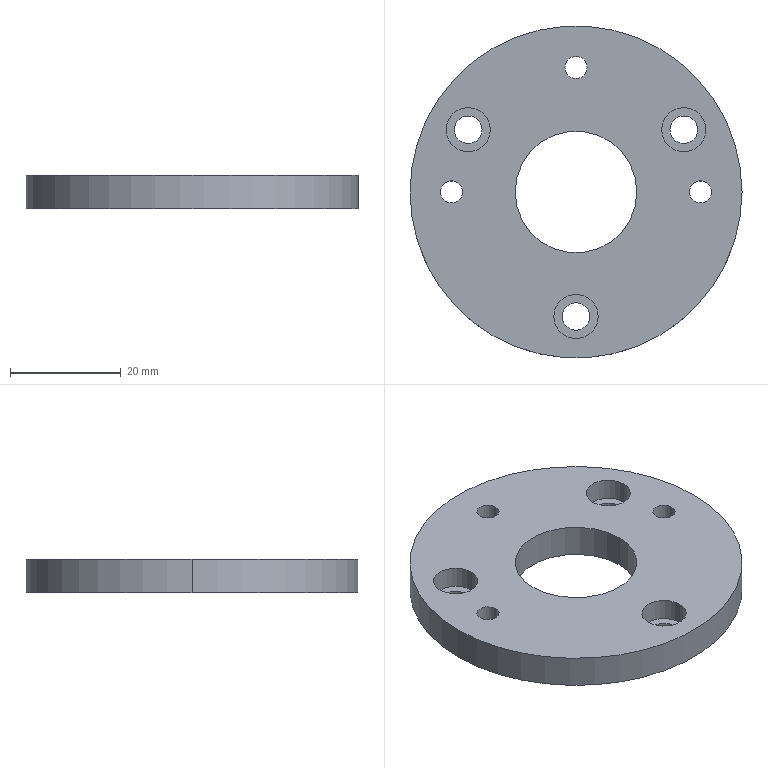Part | SolidWorks | features FlatPattern 1, ICE 1, SMBaseFlange 1, SheetMetal 1 | 1 solid | 27 faces | box 60 x 60 x 6 mm | volume 13737 mm3 | cylinder 22 | plane 5 | commonest cylinder face diameters 4 x6 5 x6 8 x6 22 x2 60 x2
STEP:
#1=CARTESIAN_POINT('',(1118.202,163.897,-4.));
#2=VERTEX_POINT('',#1);
#3=CARTESIAN_POINT('',(1126.202,163.897,-4.));
#4=VERTEX_POINT('',#3);
#5=CARTESIAN_POINT('',(1122.202,163.897,-4.));
#6=DIRECTION('',(0.,0.,1.));
#7=DIRECTION('',(1.,0.,0.));
#8=AXIS2_PLACEMENT_3D('',#5,#6,#7);
#9=CIRCLE('',#8,4.);
#10=EDGE_CURVE('',#2,#4,#9,.T.);
#11=ORIENTED_EDGE('',*,*,#10,.F.);
#12=CARTESIAN_POINT('',(1118.202,163.897,0.));
#13=VERTEX_POINT('',#12);
#14=CARTESIAN_POINT('',(1118.202,163.897,-4.));
#15=DIRECTION('',(0.,0.,1.));
#16=VECTOR('',#15,1000.);
#17=LINE('',#14,#16);
#18=EDGE_CURVE('',#2,#13,#17,.T.);
#19=ORIENTED_EDGE('',*,*,#18,.T.);
#20=CARTESIAN_POINT('',(1126.202,163.897,0.));
#21=VERTEX_POINT('',#20);
#22=CARTESIAN_POINT('',(1122.202,163.897,0.));
#23=DIRECTION('',(0.,0.,1.));
#24=DIRECTION('',(1.,0.,0.));
#25=AXIS2_PLACEMENT_3D('',#22,#23,#24);
#26=CIRCLE('',#25,4.);
#27=EDGE_CURVE('',#13,#21,#26,.T.);
#28=ORIENTED_EDGE('',*,*,#27,.T.);
#29=CARTESIAN_POINT('',(1126.202,163.897,-4.));
#30=DIRECTION('',(0.,0.,1.));
#31=VECTOR('',#30,1000.);
#32=LINE('',#29,#31);
#33=EDGE_CURVE('',#4,#21,#32,.T.);
#34=ORIENTED_EDGE('',*,*,#33,.F.);
#35=EDGE_LOOP('',(#11,#19,#28,#34));
#36=FACE_OUTER_BOUND('',#35,.T.);
#37=CARTESIAN_POINT('',(1122.202,163.897,-4.));
#38=DIRECTION('',(0.,0.,1.));
#39=DIRECTION('',(1.,0.,0.));
#40=AXIS2_PLACEMENT_3D('',#37,#38,#39);
#41=CYLINDRICAL_SURFACE('',#40,4.);
#42=ADVANCED_FACE('',(#36),#41,.F.);
#43=CARTESIAN_POINT('',(1137.687,197.647,-4.));
#44=VERTEX_POINT('',#43);
#45=CARTESIAN_POINT('',(1145.687,197.647,-4.));
#46=VERTEX_POINT('',#45);
#47=CARTESIAN_POINT('',(1141.687,197.647,-4.));
#48=DIRECTION('',(0.,0.,1.));
#49=DIRECTION('',(1.,0.,0.));
#50=AXIS2_PLACEMENT_3D('',#47,#48,#49);
#51=CIRCLE('',#50,4.);
#52=EDGE_CURVE('',#44,#46,#51,.T.);
#53=ORIENTED_EDGE('',*,*,#52,.F.);
#54=CARTESIAN_POINT('',(1137.687,197.647,0.));
#55=VERTEX_POINT('',#54);
#56=CARTESIAN_POINT('',(1137.687,197.647,-4.));
#57=DIRECTION('',(0.,0.,1.));
#58=VECTOR('',#57,1000.);
#59=LINE('',#56,#58);
#60=EDGE_CURVE('',#44,#55,#59,.T.);
#61=ORIENTED_EDGE('',*,*,#60,.T.);
#62=CARTESIAN_POINT('',(1145.687,197.647,0.));
#63=VERTEX_POINT('',#62);
#64=CARTESIAN_POINT('',(1141.687,197.647,0.));
#65=DIRECTION('',(0.,0.,1.));
#66=DIRECTION('',(1.,0.,0.));
#67=AXIS2_PLACEMENT_3D('',#64,#65,#66);
#68=CIRCLE('',#67,4.);
#69=EDGE_CURVE('',#55,#63,#68,.T.);
#70=ORIENTED_EDGE('',*,*,#69,.T.);
#71=CARTESIAN_POINT('',(1145.687,197.647,-4.));
#72=DIRECTION('',(0.,0.,1.));
#73=VECTOR('',#72,1000.);
#74=LINE('',#71,#73);
#75=EDGE_CURVE('',#46,#63,#74,.T.);
#76=ORIENTED_EDGE('',*,*,#75,.F.);
#77=EDGE_LOOP('',(#53,#61,#70,#76));
#78=FACE_OUTER_BOUND('',#77,.T.);
#79=CARTESIAN_POINT('',(1141.687,197.647,-4.));
#80=DIRECTION('',(0.,0.,1.));
#81=DIRECTION('',(1.,0.,0.));
#82=AXIS2_PLACEMENT_3D('',#79,#80,#81);
#83=CYLINDRICAL_SURFACE('',#82,4.);
#84=ADVANCED_FACE('',(#78),#83,.F.);
#85=CARTESIAN_POINT('',(1098.716,197.647,-4.));
#86=VERTEX_POINT('',#85);
#87=CARTESIAN_POINT('',(1106.716,197.647,-4.));
#88=VERTEX_POINT('',#87);
#89=CARTESIAN_POINT('',(1102.716,197.647,-4.));
#90=DIRECTION('',(0.,0.,1.));
#91=DIRECTION('',(1.,0.,0.));
#92=AXIS2_PLACEMENT_3D('',#89,#90,#91);
#93=CIRCLE('',#92,4.);
#94=EDGE_CURVE('',#86,#88,#93,.T.);
#95=ORIENTED_EDGE('',*,*,#94,.F.);
#96=CARTESIAN_POINT('',(1098.716,197.647,0.));
#97=VERTEX_POINT('',#96);
#98=CARTESIAN_POINT('',(1098.716,197.647,-4.));
#99=DIRECTION('',(0.,0.,1.));
#100=VECTOR('',#99,1000.);
#101=LINE('',#98,#100);
#102=EDGE_CURVE('',#86,#97,#101,.T.);
#103=ORIENTED_EDGE('',*,*,#102,.T.);
#104=CARTESIAN_POINT('',(1106.716,197.647,0.));
#105=VERTEX_POINT('',#104);
#106=CARTESIAN_POINT('',(1102.716,197.647,0.));
#107=DIRECTION('',(0.,0.,1.));
#108=DIRECTION('',(1.,0.,0.));
#109=AXIS2_PLACEMENT_3D('',#106,#107,#108);
#110=CIRCLE('',#109,4.);
#111=EDGE_CURVE('',#97,#105,#110,.T.);
#112=ORIENTED_EDGE('',*,*,#111,.T.);
#113=CARTESIAN_POINT('',(1106.716,197.647,-4.));
#114=DIRECTION('',(0.,0.,1.));
#115=VECTOR('',#114,1000.);
#116=LINE('',#113,#115);
#117=EDGE_CURVE('',#88,#105,#116,.T.);
#118=ORIENTED_EDGE('',*,*,#117,.F.);
#119=EDGE_LOOP('',(#95,#103,#112,#118));
#120=FACE_OUTER_BOUND('',#119,.T.);
#121=CARTESIAN_POINT('',(1102.716,197.647,-4.));
#122=DIRECTION('',(0.,0.,1.));
#123=DIRECTION('',(1.,0.,0.));
#124=AXIS2_PLACEMENT_3D('',#121,#122,#123);
#125=CYLINDRICAL_SURFACE('',#124,4.);
#126=ADVANCED_FACE('',(#120),#125,.F.);
#127=CARTESIAN_POINT('',(1142.702,186.397,-6.));
#128=VERTEX_POINT('',#127);
#129=CARTESIAN_POINT('',(1146.702,186.397,-6.));
#130=VERTEX_POINT('',#129);
#131=CARTESIAN_POINT('',(1144.702,186.397,-6.));
#132=DIRECTION('',(0.,0.,1.));
#133=DIRECTION('',(1.,0.,0.));
#134=AXIS2_PLACEMENT_3D('',#131,#132,#133);
#135=CIRCLE('',#134,2.);
#136=EDGE_CURVE('',#128,#130,#135,.T.);
#137=ORIENTED_EDGE('',*,*,#136,.F.);
#138=CARTESIAN_POINT('',(1142.702,186.397,0.));
#139=VERTEX_POINT('',#138);
#140=CARTESIAN_POINT('',(1142.702,186.397,-6.));
#141=DIRECTION('',(0.,0.,1.));
#142=VECTOR('',#141,1000.);
#143=LINE('',#140,#142);
#144=EDGE_CURVE('',#128,#139,#143,.T.);
#145=ORIENTED_EDGE('',*,*,#144,.T.);
#146=CARTESIAN_POINT('',(1146.702,186.397,0.));
#147=VERTEX_POINT('',#146);
#148=CARTESIAN_POINT('',(1144.702,186.397,0.));
#149=DIRECTION('',(0.,0.,1.));
#150=DIRECTION('',(1.,0.,0.));
#151=AXIS2_PLACEMENT_3D('',#148,#149,#150);
#152=CIRCLE('',#151,2.);
#153=EDGE_CURVE('',#139,#147,#152,.T.);
#154=ORIENTED_EDGE('',*,*,#153,.T.);
#155=CARTESIAN_POINT('',(1146.702,186.397,-6.));
#156=DIRECTION('',(0.,0.,1.));
#157=VECTOR('',#156,1000.);
#158=LINE('',#155,#157);
#159=EDGE_CURVE('',#130,#147,#158,.T.);
#160=ORIENTED_EDGE('',*,*,#159,.F.);
#161=EDGE_LOOP('',(#137,#145,#154,#160));
#162=FACE_OUTER_BOUND('',#161,.T.);
#163=CARTESIAN_POINT('',(1144.702,186.397,-6.));
#164=DIRECTION('',(0.,0.,1.));
#165=DIRECTION('',(1.,0.,0.));
#166=AXIS2_PLACEMENT_3D('',#163,#164,#165);
#167=CYLINDRICAL_SURFACE('',#166,2.);
#168=ADVANCED_FACE('',(#162),#167,.F.);
#169=CARTESIAN_POINT('',(1097.702,186.397,-6.));
#170=VERTEX_POINT('',#169);
#171=CARTESIAN_POINT('',(1101.702,186.397,-6.));
#172=VERTEX_POINT('',#171);
#173=CARTESIAN_POINT('',(1099.702,186.397,-6.));
#174=DIRECTION('',(0.,0.,1.));
#175=DIRECTION('',(1.,0.,0.));
#176=AXIS2_PLACEMENT_3D('',#173,#174,#175);
#177=CIRCLE('',#176,2.);
#178=EDGE_CURVE('',#170,#172,#177,.T.);
#179=ORIENTED_EDGE('',*,*,#178,.F.);
#180=CARTESIAN_POINT('',(1097.702,186.397,0.));
#181=VERTEX_POINT('',#180);
#182=CARTESIAN_POINT('',(1097.702,186.397,-6.));
#183=DIRECTION('',(0.,0.,1.));
#184=VECTOR('',#183,1000.);
#185=LINE('',#182,#184);
#186=EDGE_CURVE('',#170,#181,#185,.T.);
#187=ORIENTED_EDGE('',*,*,#186,.T.);
#188=CARTESIAN_POINT('',(1101.702,186.397,0.));
#189=VERTEX_POINT('',#188);
#190=CARTESIAN_POINT('',(1099.702,186.397,0.));
#191=DIRECTION('',(0.,0.,1.));
#192=DIRECTION('',(1.,0.,0.));
#193=AXIS2_PLACEMENT_3D('',#190,#191,#192);
#194=CIRCLE('',#193,2.);
#195=EDGE_CURVE('',#181,#189,#194,.T.);
#196=ORIENTED_EDGE('',*,*,#195,.T.);
#197=CARTESIAN_POINT('',(1101.702,186.397,-6.));
#198=DIRECTION('',(0.,0.,1.));
#199=VECTOR('',#198,1000.);
#200=LINE('',#197,#199);
#201=EDGE_CURVE('',#172,#189,#200,.T.);
#202=ORIENTED_EDGE('',*,*,#201,.F.);
#203=EDGE_LOOP('',(#179,#187,#196,#202));
#204=FACE_OUTER_BOUND('',#203,.T.);
#205=CARTESIAN_POINT('',(1099.702,186.397,-6.));
#206=DIRECTION('',(0.,0.,1.));
#207=DIRECTION('',(1.,0.,0.));
#208=AXIS2_PLACEMENT_3D('',#205,#206,#207);
#209=CYLINDRICAL_SURFACE('',#208,2.);
#210=ADVANCED_FACE('',(#204),#209,.F.);
#211=CARTESIAN_POINT('',(1111.202,186.397,-6.));
#212=VERTEX_POINT('',#211);
#213=CARTESIAN_POINT('',(1133.202,186.397,-6.));
#214=VERTEX_POINT('',#213);
#215=CARTESIAN_POINT('',(1122.202,186.397,-6.));
#216=DIRECTION('',(0.,0.,1.));
#217=DIRECTION('',(1.,0.,0.));
#218=AXIS2_PLACEMENT_3D('',#215,#216,#217);
#219=CIRCLE('',#218,11.);
#220=EDGE_CURVE('',#212,#214,#219,.T.);
#221=ORIENTED_EDGE('',*,*,#220,.F.);
#222=CARTESIAN_POINT('',(1111.202,186.397,0.));
#223=VERTEX_POINT('',#222);
#224=CARTESIAN_POINT('',(1111.202,186.397,-6.));
#225=DIRECTION('',(0.,0.,1.));
#226=VECTOR('',#225,1000.);
#227=LINE('',#224,#226);
#228=EDGE_CURVE('',#212,#223,#227,.T.);
#229=ORIENTED_EDGE('',*,*,#228,.T.);
#230=CARTESIAN_POINT('',(1133.202,186.397,0.));
#231=VERTEX_POINT('',#230);
#232=CARTESIAN_POINT('',(1122.202,186.397,0.));
#233=DIRECTION('',(0.,0.,1.));
#234=DIRECTION('',(1.,0.,0.));
#235=AXIS2_PLACEMENT_3D('',#232,#233,#234);
#236=CIRCLE('',#235,11.);
#237=EDGE_CURVE('',#223,#231,#236,.T.);
#238=ORIENTED_EDGE('',*,*,#237,.T.);
#239=CARTESIAN_POINT('',(1133.202,186.397,-6.));
#240=DIRECTION('',(0.,0.,1.));
#241=VECTOR('',#240,1000.);
#242=LINE('',#239,#241);
#243=EDGE_CURVE('',#214,#231,#242,.T.);
#244=ORIENTED_EDGE('',*,*,#243,.F.);
#245=EDGE_LOOP('',(#221,#229,#238,#244));
#246=FACE_OUTER_BOUND('',#245,.T.);
#247=CARTESIAN_POINT('',(1122.202,186.397,-6.));
#248=DIRECTION('',(0.,0.,1.));
#249=DIRECTION('',(1.,0.,0.));
#250=AXIS2_PLACEMENT_3D('',#247,#248,#249);
#251=CYLINDRICAL_SURFACE('',#250,11.);
#252=ADVANCED_FACE('',(#246),#251,.F.);
#253=CARTESIAN_POINT('',(1120.202,208.897,-6.));
#254=VERTEX_POINT('',#253);
#255=CARTESIAN_POINT('',(1124.202,208.897,-6.));
#256=VERTEX_POINT('',#255);
#257=CARTESIAN_POINT('',(1122.202,208.897,-6.));
#258=DIRECTION('',(0.,0.,1.));
#259=DIRECTION('',(1.,0.,0.));
#260=AXIS2_PLACEMENT_3D('',#257,#258,#259);
#261=CIRCLE('',#260,2.);
#262=EDGE_CURVE('',#254,#256,#261,.T.);
#263=ORIENTED_EDGE('',*,*,#262,.F.);
#264=CARTESIAN_POINT('',(1120.202,208.897,0.));
#265=VERTEX_POINT('',#264);
#266=CARTESIAN_POINT('',(1120.202,208.897,-6.));
#267=DIRECTION('',(0.,0.,1.));
#268=VECTOR('',#267,1000.);
#269=LINE('',#266,#268);
#270=EDGE_CURVE('',#254,#265,#269,.T.);
#271=ORIENTED_EDGE('',*,*,#270,.T.);
#272=CARTESIAN_POINT('',(1124.202,208.897,0.));
#273=VERTEX_POINT('',#272);
#274=CARTESIAN_POINT('',(1122.202,208.897,0.));
#275=DIRECTION('',(0.,0.,1.));
#276=DIRECTION('',(1.,0.,0.));
#277=AXIS2_PLACEMENT_3D('',#274,#275,#276);
#278=CIRCLE('',#277,2.);
#279=EDGE_CURVE('',#265,#273,#278,.T.);
#280=ORIENTED_EDGE('',*,*,#279,.T.);
#281=CARTESIAN_POINT('',(1124.202,208.897,-6.));
#282=DIRECTION('',(0.,0.,1.));
#283=VECTOR('',#282,1000.);
#284=LINE('',#281,#283);
#285=EDGE_CURVE('',#256,#273,#284,.T.);
#286=ORIENTED_EDGE('',*,*,#285,.F.);
#287=EDGE_LOOP('',(#263,#271,#280,#286));
#288=FACE_OUTER_BOUND('',#287,.T.);
#289=CARTESIAN_POINT('',(1122.202,208.897,-6.));
#290=DIRECTION('',(0.,0.,1.));
#291=DIRECTION('',(1.,0.,0.));
#292=AXIS2_PLACEMENT_3D('',#289,#290,#291);
#293=CYLINDRICAL_SURFACE('',#292,2.);
#294=ADVANCED_FACE('',(#288),#293,.F.);
#295=CARTESIAN_POINT('',(1152.202,186.397,-6.));
#296=VERTEX_POINT('',#295);
#297=CARTESIAN_POINT('',(1092.202,186.397,-6.));
#298=VERTEX_POINT('',#297);
#299=CARTESIAN_POINT('',(1122.202,186.397,-6.));
#300=DIRECTION('',(0.,0.,1.));
#301=DIRECTION('',(1.,0.,0.));
#302=AXIS2_PLACEMENT_3D('',#299,#300,#301);
#303=CIRCLE('',#302,30.);
#304=EDGE_CURVE('',#296,#298,#303,.T.);
#305=ORIENTED_EDGE('',*,*,#304,.T.);
#306=CARTESIAN_POINT('',(1092.202,186.397,0.));
#307=VERTEX_POINT('',#306);
#308=CARTESIAN_POINT('',(1092.202,186.397,-6.));
#309=DIRECTION('',(0.,0.,1.));
#310=VECTOR('',#309,1000.);
#311=LINE('',#308,#310);
#312=EDGE_CURVE('',#298,#307,#311,.T.);
#313=ORIENTED_EDGE('',*,*,#312,.T.);
#314=CARTESIAN_POINT('',(1152.202,186.397,0.));
#315=VERTEX_POINT('',#314);
#316=CARTESIAN_POINT('',(1122.202,186.397,0.));
#317=DIRECTION('',(0.,0.,1.));
#318=DIRECTION('',(1.,0.,0.));
#319=AXIS2_PLACEMENT_3D('',#316,#317,#318);
#320=CIRCLE('',#319,30.);
#321=EDGE_CURVE('',#315,#307,#320,.T.);
#322=ORIENTED_EDGE('',*,*,#321,.F.);
#323=CARTESIAN_POINT('',(1152.202,186.397,-6.));
#324=DIRECTION('',(0.,0.,1.));
#325=VECTOR('',#324,1000.);
#326=LINE('',#323,#325);
#327=EDGE_CURVE('',#296,#315,#326,.T.);
#328=ORIENTED_EDGE('',*,*,#327,.F.);
#329=EDGE_LOOP('',(#305,#313,#322,#328));
#330=FACE_OUTER_BOUND('',#329,.T.);
#331=CARTESIAN_POINT('',(1122.202,186.397,-6.));
#332=DIRECTION('',(0.,0.,1.));
#333=DIRECTION('',(1.,0.,0.));
#334=AXIS2_PLACEMENT_3D('',#331,#332,#333);
#335=CYLINDRICAL_SURFACE('',#334,30.);
#336=ADVANCED_FACE('',(#330),#335,.T.);
#337=CARTESIAN_POINT('',(1100.216,197.647,-6.));
#338=VERTEX_POINT('',#337);
#339=CARTESIAN_POINT('',(1105.216,197.647,-6.));
#340=VERTEX_POINT('',#339);
#341=CARTESIAN_POINT('',(1102.716,197.647,-6.));
#342=DIRECTION('',(0.,0.,1.));
#343=DIRECTION('',(1.,0.,0.));
#344=AXIS2_PLACEMENT_3D('',#341,#342,#343);
#345=CIRCLE('',#344,2.5);
#346=EDGE_CURVE('',#338,#340,#345,.T.);
#347=ORIENTED_EDGE('',*,*,#346,.F.);
#348=CARTESIAN_POINT('',(1100.216,197.647,-4.));
#349=VERTEX_POINT('',#348);
#350=CARTESIAN_POINT('',(1100.216,197.647,-6.));
#351=DIRECTION('',(0.,0.,1.));
#352=VECTOR('',#351,1000.);
#353=LINE('',#350,#352);
#354=EDGE_CURVE('',#338,#349,#353,.T.);
#355=ORIENTED_EDGE('',*,*,#354,.T.);
#356=CARTESIAN_POINT('',(1105.216,197.647,-4.));
#357=VERTEX_POINT('',#356);
#358=CARTESIAN_POINT('',(1102.716,197.647,-4.));
#359=DIRECTION('',(0.,0.,-1.));
#360=DIRECTION('',(1.,0.,0.));
#361=AXIS2_PLACEMENT_3D('',#358,#359,#360);
#362=CIRCLE('',#361,2.5);
#363=EDGE_CURVE('',#357,#349,#362,.T.);
#364=ORIENTED_EDGE('',*,*,#363,.F.);
#365=CARTESIAN_POINT('',(1105.216,197.647,-6.));
#366=DIRECTION('',(0.,0.,1.));
#367=VECTOR('',#366,1000.);
#368=LINE('',#365,#367);
#369=EDGE_CURVE('',#340,#357,#368,.T.);
#370=ORIENTED_EDGE('',*,*,#369,.F.);
#371=EDGE_LOOP('',(#347,#355,#364,#370));
#372=FACE_OUTER_BOUND('',#371,.T.);
#373=CARTESIAN_POINT('',(1102.716,197.647,-6.));
#374=DIRECTION('',(0.,0.,1.));
#375=DIRECTION('',(1.,0.,0.));
#376=AXIS2_PLACEMENT_3D('',#373,#374,#375);
#377=CYLINDRICAL_SURFACE('',#376,2.5);
#378=ADVANCED_FACE('',(#372),#377,.F.);
#379=CARTESIAN_POINT('',(1139.187,197.647,-6.));
#380=VERTEX_POINT('',#379);
#381=CARTESIAN_POINT('',(1144.187,197.647,-6.));
#382=VERTEX_POINT('',#381);
#383=CARTESIAN_POINT('',(1141.687,197.647,-6.));
#384=DIRECTION('',(0.,0.,1.));
#385=DIRECTION('',(1.,0.,0.));
#386=AXIS2_PLACEMENT_3D('',#383,#384,#385);
#387=CIRCLE('',#386,2.5);
#388=EDGE_CURVE('',#380,#382,#387,.T.);
#389=ORIENTED_EDGE('',*,*,#388,.F.);
#390=CARTESIAN_POINT('',(1139.187,197.647,-4.));
#391=VERTEX_POINT('',#390);
#392=CARTESIAN_POINT('',(1139.187,197.647,-6.));
#393=DIRECTION('',(0.,0.,1.));
#394=VECTOR('',#393,1000.);
#395=LINE('',#392,#394);
#396=EDGE_CURVE('',#380,#391,#395,.T.);
#397=ORIENTED_EDGE('',*,*,#396,.T.);
#398=CARTESIAN_POINT('',(1144.187,197.647,-4.));
#399=VERTEX_POINT('',#398);
#400=CARTESIAN_POINT('',(1141.687,197.647,-4.));
#401=DIRECTION('',(0.,0.,-1.));
#402=DIRECTION('',(1.,0.,0.));
#403=AXIS2_PLACEMENT_3D('',#400,#401,#402);
#404=CIRCLE('',#403,2.5);
#405=EDGE_CURVE('',#399,#391,#404,.T.);
#406=ORIENTED_EDGE('',*,*,#405,.F.);
#407=CARTESIAN_POINT('',(1144.187,197.647,-6.));
#408=DIRECTION('',(0.,0.,1.));
#409=VECTOR('',#408,1000.);
#410=LINE('',#407,#409);
#411=EDGE_CURVE('',#382,#399,#410,.T.);
#412=ORIENTED_EDGE('',*,*,#411,.F.);
#413=EDGE_LOOP('',(#389,#397,#406,#412));
#414=FACE_OUTER_BOUND('',#413,.T.);
#415=CARTESIAN_POINT('',(1141.687,197.647,-6.));
#416=DIRECTION('',(0.,0.,1.));
#417=DIRECTION('',(1.,0.,0.));
#418=AXIS2_PLACEMENT_3D('',#415,#416,#417);
#419=CYLINDRICAL_SURFACE('',#418,2.5);
#420=ADVANCED_FACE('',(#414),#419,.F.);
#421=CARTESIAN_POINT('',(1119.702,163.897,-6.));
#422=VERTEX_POINT('',#421);
#423=CARTESIAN_POINT('',(1124.702,163.897,-6.));
#424=VERTEX_POINT('',#423);
#425=CARTESIAN_POINT('',(1122.202,163.897,-6.));
#426=DIRECTION('',(0.,0.,1.));
#427=DIRECTION('',(1.,0.,0.));
#428=AXIS2_PLACEMENT_3D('',#425,#426,#427);
#429=CIRCLE('',#428,2.5);
#430=EDGE_CURVE('',#422,#424,#429,.T.);
#431=ORIENTED_EDGE('',*,*,#430,.F.);
#432=CARTESIAN_POINT('',(1119.702,163.897,-4.));
#433=VERTEX_POINT('',#432);
#434=CARTESIAN_POINT('',(1119.702,163.897,-6.));
#435=DIRECTION('',(0.,0.,1.));
#436=VECTOR('',#435,1000.);
#437=LINE('',#434,#436);
#438=EDGE_CURVE('',#422,#433,#437,.T.);
#439=ORIENTED_EDGE('',*,*,#438,.T.);
#440=CARTESIAN_POINT('',(1124.702,163.897,-4.));
#441=VERTEX_POINT('',#440);
#442=CARTESIAN_POINT('',(1122.202,163.897,-4.));
#443=DIRECTION('',(0.,0.,-1.));
#444=DIRECTION('',(1.,0.,0.));
#445=AXIS2_PLACEMENT_3D('',#442,#443,#444);
#446=CIRCLE('',#445,2.5);
#447=EDGE_CURVE('',#441,#433,#446,.T.);
#448=ORIENTED_EDGE('',*,*,#447,.F.);
#449=CARTESIAN_POINT('',(1124.702,163.897,-6.));
#450=DIRECTION('',(0.,0.,1.));
#451=VECTOR('',#450,1000.);
#452=LINE('',#449,#451);
#453=EDGE_CURVE('',#424,#441,#452,.T.);
#454=ORIENTED_EDGE('',*,*,#453,.F.);
#455=EDGE_LOOP('',(#431,#439,#448,#454));
#456=FACE_OUTER_BOUND('',#455,.T.);
#457=CARTESIAN_POINT('',(1122.202,163.897,-6.));
#458=DIRECTION('',(0.,0.,1.));
#459=DIRECTION('',(1.,0.,0.));
#460=AXIS2_PLACEMENT_3D('',#457,#458,#459);
#461=CYLINDRICAL_SURFACE('',#460,2.5);
#462=ADVANCED_FACE('',(#456),#461,.F.);
#463=ORIENTED_EDGE('',*,*,#438,.F.);
#464=CARTESIAN_POINT('',(1122.202,163.897,-6.));
#465=DIRECTION('',(0.,0.,1.));
#466=DIRECTION('',(1.,0.,0.));
#467=AXIS2_PLACEMENT_3D('',#464,#465,#466);
#468=CIRCLE('',#467,2.5);
#469=EDGE_CURVE('',#424,#422,#468,.T.);
#470=ORIENTED_EDGE('',*,*,#469,.F.);
#471=ORIENTED_EDGE('',*,*,#453,.T.);
#472=CARTESIAN_POINT('',(1122.202,163.897,-4.));
#473=DIRECTION('',(0.,0.,-1.));
#474=DIRECTION('',(1.,0.,0.));
#475=AXIS2_PLACEMENT_3D('',#472,#473,#474);
#476=CIRCLE('',#475,2.5);
#477=EDGE_CURVE('',#433,#441,#476,.T.);
#478=ORIENTED_EDGE('',*,*,#477,.F.);
#479=EDGE_LOOP('',(#463,#470,#471,#478));
#480=FACE_OUTER_BOUND('',#479,.T.);
#481=CARTESIAN_POINT('',(1122.202,163.897,-6.));
#482=DIRECTION('',(0.,0.,1.));
#483=DIRECTION('',(1.,0.,0.));
#484=AXIS2_PLACEMENT_3D('',#481,#482,#483);
#485=CYLINDRICAL_SURFACE('',#484,2.5);
#486=ADVANCED_FACE('',(#480),#485,.F.);
#487=ORIENTED_EDGE('',*,*,#396,.F.);
#488=CARTESIAN_POINT('',(1141.687,197.647,-6.));
#489=DIRECTION('',(0.,0.,1.));
#490=DIRECTION('',(1.,0.,0.));
#491=AXIS2_PLACEMENT_3D('',#488,#489,#490);
#492=CIRCLE('',#491,2.5);
#493=EDGE_CURVE('',#382,#380,#492,.T.);
#494=ORIENTED_EDGE('',*,*,#493,.F.);
#495=ORIENTED_EDGE('',*,*,#411,.T.);
#496=CARTESIAN_POINT('',(1141.687,197.647,-4.));
#497=DIRECTION('',(0.,0.,-1.));
#498=DIRECTION('',(1.,0.,0.));
#499=AXIS2_PLACEMENT_3D('',#496,#497,#498);
#500=CIRCLE('',#499,2.5);
#501=EDGE_CURVE('',#391,#399,#500,.T.);
#502=ORIENTED_EDGE('',*,*,#501,.F.);
#503=EDGE_LOOP('',(#487,#494,#495,#502));
#504=FACE_OUTER_BOUND('',#503,.T.);
#505=CARTESIAN_POINT('',(1141.687,197.647,-6.));
#506=DIRECTION('',(0.,0.,1.));
#507=DIRECTION('',(1.,0.,0.));
#508=AXIS2_PLACEMENT_3D('',#505,#506,#507);
#509=CYLINDRICAL_SURFACE('',#508,2.5);
#510=ADVANCED_FACE('',(#504),#509,.F.);
#511=ORIENTED_EDGE('',*,*,#354,.F.);
#512=CARTESIAN_POINT('',(1102.716,197.647,-6.));
#513=DIRECTION('',(0.,0.,1.));
#514=DIRECTION('',(1.,0.,0.));
#515=AXIS2_PLACEMENT_3D('',#512,#513,#514);
#516=CIRCLE('',#515,2.5);
#517=EDGE_CURVE('',#340,#338,#516,.T.);
#518=ORIENTED_EDGE('',*,*,#517,.F.);
#519=ORIENTED_EDGE('',*,*,#369,.T.);
#520=CARTESIAN_POINT('',(1102.716,197.647,-4.));
#521=DIRECTION('',(0.,0.,-1.));
#522=DIRECTION('',(1.,0.,0.));
#523=AXIS2_PLACEMENT_3D('',#520,#521,#522);
#524=CIRCLE('',#523,2.5);
#525=EDGE_CURVE('',#349,#357,#524,.T.);
#526=ORIENTED_EDGE('',*,*,#525,.F.);
#527=EDGE_LOOP('',(#511,#518,#519,#526));
#528=FACE_OUTER_BOUND('',#527,.T.);
#529=CARTESIAN_POINT('',(1102.716,197.647,-6.));
#530=DIRECTION('',(0.,0.,1.));
#531=DIRECTION('',(1.,0.,0.));
#532=AXIS2_PLACEMENT_3D('',#529,#530,#531);
#533=CYLINDRICAL_SURFACE('',#532,2.5);
#534=ADVANCED_FACE('',(#528),#533,.F.);
#535=ORIENTED_EDGE('',*,*,#312,.F.);
#536=CARTESIAN_POINT('',(1122.202,186.397,-6.));
#537=DIRECTION('',(0.,0.,1.));
#538=DIRECTION('',(1.,0.,0.));
#539=AXIS2_PLACEMENT_3D('',#536,#537,#538);
#540=CIRCLE('',#539,30.);
#541=EDGE_CURVE('',#298,#296,#540,.T.);
#542=ORIENTED_EDGE('',*,*,#541,.T.);
#543=ORIENTED_EDGE('',*,*,#327,.T.);
#544=CARTESIAN_POINT('',(1122.202,186.397,0.));
#545=DIRECTION('',(0.,0.,1.));
#546=DIRECTION('',(1.,0.,0.));
#547=AXIS2_PLACEMENT_3D('',#544,#545,#546);
#548=CIRCLE('',#547,30.);
#549=EDGE_CURVE('',#307,#315,#548,.T.);
#550=ORIENTED_EDGE('',*,*,#549,.F.);
#551=EDGE_LOOP('',(#535,#542,#543,#550));
#552=FACE_OUTER_BOUND('',#551,.T.);
#553=CARTESIAN_POINT('',(1122.202,186.397,-6.));
#554=DIRECTION('',(0.,0.,1.));
#555=DIRECTION('',(1.,0.,0.));
#556=AXIS2_PLACEMENT_3D('',#553,#554,#555);
#557=CYLINDRICAL_SURFACE('',#556,30.);
#558=ADVANCED_FACE('',(#552),#557,.T.);
#559=CARTESIAN_POINT('',(1144.702,186.397,-6.));
#560=DIRECTION('',(0.,0.,1.));
#561=DIRECTION('',(1.,0.,0.));
#562=AXIS2_PLACEMENT_3D('',#559,#560,#561);
#563=CIRCLE('',#562,2.);
#564=EDGE_CURVE('',#130,#128,#563,.T.);
#565=ORIENTED_EDGE('',*,*,#564,.T.);
#566=ORIENTED_EDGE('',*,*,#136,.T.);
#567=EDGE_LOOP('',(#565,#566));
#568=FACE_BOUND('',#567,.T.);
#569=CARTESIAN_POINT('',(1099.702,186.397,-6.));
#570=DIRECTION('',(0.,0.,1.));
#571=DIRECTION('',(1.,0.,0.));
#572=AXIS2_PLACEMENT_3D('',#569,#570,#571);
#573=CIRCLE('',#572,2.);
#574=EDGE_CURVE('',#172,#170,#573,.T.);
#575=ORIENTED_EDGE('',*,*,#574,.T.);
#576=ORIENTED_EDGE('',*,*,#178,.T.);
#577=EDGE_LOOP('',(#575,#576));
#578=FACE_BOUND('',#577,.T.);
#579=ORIENTED_EDGE('',*,*,#493,.T.);
#580=ORIENTED_EDGE('',*,*,#388,.T.);
#581=EDGE_LOOP('',(#579,#580));
#582=FACE_BOUND('',#581,.T.);
#583=ORIENTED_EDGE('',*,*,#517,.T.);
#584=ORIENTED_EDGE('',*,*,#346,.T.);
#585=EDGE_LOOP('',(#583,#584));
#586=FACE_BOUND('',#585,.T.);
#587=CARTESIAN_POINT('',(1122.202,186.397,-6.));
#588=DIRECTION('',(0.,0.,1.));
#589=DIRECTION('',(1.,0.,0.));
#590=AXIS2_PLACEMENT_3D('',#587,#588,#589);
#591=CIRCLE('',#590,11.);
#592=EDGE_CURVE('',#214,#212,#591,.T.);
#593=ORIENTED_EDGE('',*,*,#592,.T.);
#594=ORIENTED_EDGE('',*,*,#220,.T.);
#595=EDGE_LOOP('',(#593,#594));
#596=FACE_BOUND('',#595,.T.);
#597=CARTESIAN_POINT('',(1122.202,208.897,-6.));
#598=DIRECTION('',(0.,0.,1.));
#599=DIRECTION('',(1.,0.,0.));
#600=AXIS2_PLACEMENT_3D('',#597,#598,#599);
#601=CIRCLE('',#600,2.);
#602=EDGE_CURVE('',#256,#254,#601,.T.);
#603=ORIENTED_EDGE('',*,*,#602,.T.);
#604=ORIENTED_EDGE('',*,*,#262,.T.);
#605=EDGE_LOOP('',(#603,#604));
#606=FACE_BOUND('',#605,.T.);
#607=ORIENTED_EDGE('',*,*,#469,.T.);
#608=ORIENTED_EDGE('',*,*,#430,.T.);
#609=EDGE_LOOP('',(#607,#608));
#610=FACE_BOUND('',#609,.T.);
#611=ORIENTED_EDGE('',*,*,#304,.F.);
#612=ORIENTED_EDGE('',*,*,#541,.F.);
#613=EDGE_LOOP('',(#611,#612));
#614=FACE_OUTER_BOUND('',#613,.T.);
#615=CARTESIAN_POINT('',(1122.202,186.397,-6.));
#616=DIRECTION('',(0.,0.,1.));
#617=DIRECTION('',(1.,0.,0.));
#618=AXIS2_PLACEMENT_3D('',#615,#616,#617);
#619=PLANE('',#618);
#620=ADVANCED_FACE('',(#568,#578,#582,#586,#596,#606,#610,#614),#619,.F.);
#621=CARTESIAN_POINT('',(1122.202,163.897,0.));
#622=DIRECTION('',(0.,0.,1.));
#623=DIRECTION('',(1.,0.,0.));
#624=AXIS2_PLACEMENT_3D('',#621,#622,#623);
#625=CIRCLE('',#624,4.);
#626=EDGE_CURVE('',#21,#13,#625,.T.);
#627=ORIENTED_EDGE('',*,*,#626,.F.);
#628=ORIENTED_EDGE('',*,*,#27,.F.);
#629=EDGE_LOOP('',(#627,#628));
#630=FACE_BOUND('',#629,.T.);
#631=CARTESIAN_POINT('',(1141.687,197.647,0.));
#632=DIRECTION('',(0.,0.,1.));
#633=DIRECTION('',(1.,0.,0.));
#634=AXIS2_PLACEMENT_3D('',#631,#632,#633);
#635=CIRCLE('',#634,4.);
#636=EDGE_CURVE('',#63,#55,#635,.T.);
#637=ORIENTED_EDGE('',*,*,#636,.F.);
#638=ORIENTED_EDGE('',*,*,#69,.F.);
#639=EDGE_LOOP('',(#637,#638));
#640=FACE_BOUND('',#639,.T.);
#641=CARTESIAN_POINT('',(1102.716,197.647,0.));
#642=DIRECTION('',(0.,0.,1.));
#643=DIRECTION('',(1.,0.,0.));
#644=AXIS2_PLACEMENT_3D('',#641,#642,#643);
#645=CIRCLE('',#644,4.);
#646=EDGE_CURVE('',#105,#97,#645,.T.);
#647=ORIENTED_EDGE('',*,*,#646,.F.);
#648=ORIENTED_EDGE('',*,*,#111,.F.);
#649=EDGE_LOOP('',(#647,#648));
#650=FACE_BOUND('',#649,.T.);
#651=CARTESIAN_POINT('',(1144.702,186.397,0.));
#652=DIRECTION('',(0.,0.,1.));
#653=DIRECTION('',(1.,0.,0.));
#654=AXIS2_PLACEMENT_3D('',#651,#652,#653);
#655=CIRCLE('',#654,2.);
#656=EDGE_CURVE('',#147,#139,#655,.T.);
#657=ORIENTED_EDGE('',*,*,#656,.F.);
#658=ORIENTED_EDGE('',*,*,#153,.F.);
#659=EDGE_LOOP('',(#657,#658));
#660=FACE_BOUND('',#659,.T.);
#661=CARTESIAN_POINT('',(1099.702,186.397,0.));
#662=DIRECTION('',(0.,0.,1.));
#663=DIRECTION('',(1.,0.,0.));
#664=AXIS2_PLACEMENT_3D('',#661,#662,#663);
#665=CIRCLE('',#664,2.);
#666=EDGE_CURVE('',#189,#181,#665,.T.);
#667=ORIENTED_EDGE('',*,*,#666,.F.);
#668=ORIENTED_EDGE('',*,*,#195,.F.);
#669=EDGE_LOOP('',(#667,#668));
#670=FACE_BOUND('',#669,.T.);
#671=CARTESIAN_POINT('',(1122.202,186.397,0.));
#672=DIRECTION('',(0.,0.,1.));
#673=DIRECTION('',(1.,0.,0.));
#674=AXIS2_PLACEMENT_3D('',#671,#672,#673);
#675=CIRCLE('',#674,11.);
#676=EDGE_CURVE('',#231,#223,#675,.T.);
#677=ORIENTED_EDGE('',*,*,#676,.F.);
#678=ORIENTED_EDGE('',*,*,#237,.F.);
#679=EDGE_LOOP('',(#677,#678));
#680=FACE_BOUND('',#679,.T.);
#681=CARTESIAN_POINT('',(1122.202,208.897,0.));
#682=DIRECTION('',(0.,0.,1.));
#683=DIRECTION('',(1.,0.,0.));
#684=AXIS2_PLACEMENT_3D('',#681,#682,#683);
#685=CIRCLE('',#684,2.);
#686=EDGE_CURVE('',#273,#265,#685,.T.);
#687=ORIENTED_EDGE('',*,*,#686,.F.);
#688=ORIENTED_EDGE('',*,*,#279,.F.);
#689=EDGE_LOOP('',(#687,#688));
#690=FACE_BOUND('',#689,.T.);
#691=ORIENTED_EDGE('',*,*,#321,.T.);
#692=ORIENTED_EDGE('',*,*,#549,.T.);
#693=EDGE_LOOP('',(#691,#692));
#694=FACE_OUTER_BOUND('',#693,.T.);
#695=CARTESIAN_POINT('',(1122.202,186.397,0.));
#696=DIRECTION('',(0.,0.,1.));
#697=DIRECTION('',(1.,0.,0.));
#698=AXIS2_PLACEMENT_3D('',#695,#696,#697);
#699=PLANE('',#698);
#700=ADVANCED_FACE('',(#630,#640,#650,#660,#670,#680,#690,#694),#699,.T.);
#701=ORIENTED_EDGE('',*,*,#270,.F.);
#702=ORIENTED_EDGE('',*,*,#602,.F.);
#703=ORIENTED_EDGE('',*,*,#285,.T.);
#704=ORIENTED_EDGE('',*,*,#686,.T.);
#705=EDGE_LOOP('',(#701,#702,#703,#704));
#706=FACE_OUTER_BOUND('',#705,.T.);
#707=CARTESIAN_POINT('',(1122.202,208.897,-6.));
#708=DIRECTION('',(0.,0.,1.));
#709=DIRECTION('',(1.,0.,0.));
#710=AXIS2_PLACEMENT_3D('',#707,#708,#709);
#711=CYLINDRICAL_SURFACE('',#710,2.);
#712=ADVANCED_FACE('',(#706),#711,.F.);
#713=ORIENTED_EDGE('',*,*,#228,.F.);
#714=ORIENTED_EDGE('',*,*,#592,.F.);
#715=ORIENTED_EDGE('',*,*,#243,.T.);
#716=ORIENTED_EDGE('',*,*,#676,.T.);
#717=EDGE_LOOP('',(#713,#714,#715,#716));
#718=FACE_OUTER_BOUND('',#717,.T.);
#719=CARTESIAN_POINT('',(1122.202,186.397,-6.));
#720=DIRECTION('',(0.,0.,1.));
#721=DIRECTION('',(1.,0.,0.));
#722=AXIS2_PLACEMENT_3D('',#719,#720,#721);
#723=CYLINDRICAL_SURFACE('',#722,11.);
#724=ADVANCED_FACE('',(#718),#723,.F.);
#725=ORIENTED_EDGE('',*,*,#186,.F.);
#726=ORIENTED_EDGE('',*,*,#574,.F.);
#727=ORIENTED_EDGE('',*,*,#201,.T.);
#728=ORIENTED_EDGE('',*,*,#666,.T.);
#729=EDGE_LOOP('',(#725,#726,#727,#728));
#730=FACE_OUTER_BOUND('',#729,.T.);
#731=CARTESIAN_POINT('',(1099.702,186.397,-6.));
#732=DIRECTION('',(0.,0.,1.));
#733=DIRECTION('',(1.,0.,0.));
#734=AXIS2_PLACEMENT_3D('',#731,#732,#733);
#735=CYLINDRICAL_SURFACE('',#734,2.);
#736=ADVANCED_FACE('',(#730),#735,.F.);
#737=ORIENTED_EDGE('',*,*,#144,.F.);
#738=ORIENTED_EDGE('',*,*,#564,.F.);
#739=ORIENTED_EDGE('',*,*,#159,.T.);
#740=ORIENTED_EDGE('',*,*,#656,.T.);
#741=EDGE_LOOP('',(#737,#738,#739,#740));
#742=FACE_OUTER_BOUND('',#741,.T.);
#743=CARTESIAN_POINT('',(1144.702,186.397,-6.));
#744=DIRECTION('',(0.,0.,1.));
#745=DIRECTION('',(1.,0.,0.));
#746=AXIS2_PLACEMENT_3D('',#743,#744,#745);
#747=CYLINDRICAL_SURFACE('',#746,2.);
#748=ADVANCED_FACE('',(#742),#747,.F.);
#749=CARTESIAN_POINT('',(1102.716,197.647,-4.));
#750=DIRECTION('',(0.,0.,1.));
#751=DIRECTION('',(1.,0.,0.));
#752=AXIS2_PLACEMENT_3D('',#749,#750,#751);
#753=CIRCLE('',#752,4.);
#754=EDGE_CURVE('',#88,#86,#753,.T.);
#755=ORIENTED_EDGE('',*,*,#754,.T.);
#756=ORIENTED_EDGE('',*,*,#94,.T.);
#757=EDGE_LOOP('',(#755,#756));
#758=FACE_OUTER_BOUND('',#757,.T.);
#759=ORIENTED_EDGE('',*,*,#363,.T.);
#760=ORIENTED_EDGE('',*,*,#525,.T.);
#761=EDGE_LOOP('',(#759,#760));
#762=FACE_BOUND('',#761,.T.);
#763=CARTESIAN_POINT('',(1102.716,197.647,-4.));
#764=DIRECTION('',(0.,0.,1.));
#765=DIRECTION('',(1.,0.,0.));
#766=AXIS2_PLACEMENT_3D('',#763,#764,#765);
#767=PLANE('',#766);
#768=ADVANCED_FACE('',(#758,#762),#767,.T.);
#769=ORIENTED_EDGE('',*,*,#102,.F.);
#770=ORIENTED_EDGE('',*,*,#754,.F.);
#771=ORIENTED_EDGE('',*,*,#117,.T.);
#772=ORIENTED_EDGE('',*,*,#646,.T.);
#773=EDGE_LOOP('',(#769,#770,#771,#772));
#774=FACE_OUTER_BOUND('',#773,.T.);
#775=CARTESIAN_POINT('',(1102.716,197.647,-4.));
#776=DIRECTION('',(0.,0.,1.));
#777=DIRECTION('',(1.,0.,0.));
#778=AXIS2_PLACEMENT_3D('',#775,#776,#777);
#779=CYLINDRICAL_SURFACE('',#778,4.);
#780=ADVANCED_FACE('',(#774),#779,.F.);
#781=CARTESIAN_POINT('',(1141.687,197.647,-4.));
#782=DIRECTION('',(0.,0.,1.));
#783=DIRECTION('',(1.,0.,0.));
#784=AXIS2_PLACEMENT_3D('',#781,#782,#783);
#785=CIRCLE('',#784,4.);
#786=EDGE_CURVE('',#46,#44,#785,.T.);
#787=ORIENTED_EDGE('',*,*,#786,.T.);
#788=ORIENTED_EDGE('',*,*,#52,.T.);
#789=EDGE_LOOP('',(#787,#788));
#790=FACE_OUTER_BOUND('',#789,.T.);
#791=ORIENTED_EDGE('',*,*,#405,.T.);
#792=ORIENTED_EDGE('',*,*,#501,.T.);
#793=EDGE_LOOP('',(#791,#792));
#794=FACE_BOUND('',#793,.T.);
#795=CARTESIAN_POINT('',(1141.687,197.647,-4.));
#796=DIRECTION('',(0.,0.,1.));
#797=DIRECTION('',(1.,0.,0.));
#798=AXIS2_PLACEMENT_3D('',#795,#796,#797);
#799=PLANE('',#798);
#800=ADVANCED_FACE('',(#790,#794),#799,.T.);
#801=ORIENTED_EDGE('',*,*,#60,.F.);
#802=ORIENTED_EDGE('',*,*,#786,.F.);
#803=ORIENTED_EDGE('',*,*,#75,.T.);
#804=ORIENTED_EDGE('',*,*,#636,.T.);
#805=EDGE_LOOP('',(#801,#802,#803,#804));
#806=FACE_OUTER_BOUND('',#805,.T.);
#807=CARTESIAN_POINT('',(1141.687,197.647,-4.));
#808=DIRECTION('',(0.,0.,1.));
#809=DIRECTION('',(1.,0.,0.));
#810=AXIS2_PLACEMENT_3D('',#807,#808,#809);
#811=CYLINDRICAL_SURFACE('',#810,4.);
#812=ADVANCED_FACE('',(#806),#811,.F.);
#813=CARTESIAN_POINT('',(1122.202,163.897,-4.));
#814=DIRECTION('',(0.,0.,1.));
#815=DIRECTION('',(1.,0.,0.));
#816=AXIS2_PLACEMENT_3D('',#813,#814,#815);
#817=CIRCLE('',#816,4.);
#818=EDGE_CURVE('',#4,#2,#817,.T.);
#819=ORIENTED_EDGE('',*,*,#818,.T.);
#820=ORIENTED_EDGE('',*,*,#10,.T.);
#821=EDGE_LOOP('',(#819,#820));
#822=FACE_OUTER_BOUND('',#821,.T.);
#823=ORIENTED_EDGE('',*,*,#447,.T.);
#824=ORIENTED_EDGE('',*,*,#477,.T.);
#825=EDGE_LOOP('',(#823,#824));
#826=FACE_BOUND('',#825,.T.);
#827=CARTESIAN_POINT('',(1122.202,163.897,-4.));
#828=DIRECTION('',(0.,0.,1.));
#829=DIRECTION('',(1.,0.,0.));
#830=AXIS2_PLACEMENT_3D('',#827,#828,#829);
#831=PLANE('',#830);
#832=ADVANCED_FACE('',(#822,#826),#831,.T.);
#833=ORIENTED_EDGE('',*,*,#18,.F.);
#834=ORIENTED_EDGE('',*,*,#818,.F.);
#835=ORIENTED_EDGE('',*,*,#33,.T.);
#836=ORIENTED_EDGE('',*,*,#626,.T.);
#837=EDGE_LOOP('',(#833,#834,#835,#836));
#838=FACE_OUTER_BOUND('',#837,.T.);
#839=CARTESIAN_POINT('',(1122.202,163.897,-4.));
#840=DIRECTION('',(0.,0.,1.));
#841=DIRECTION('',(1.,0.,0.));
#842=AXIS2_PLACEMENT_3D('',#839,#840,#841);
#843=CYLINDRICAL_SURFACE('',#842,4.);
#844=ADVANCED_FACE('',(#838),#843,.F.);
#845=CLOSED_SHELL('',(#42,#84,#126,#168,#210,#252,#294,#336,#378,#420,#462,#486,#510,#534,#558,#620,#700,#712,#724,#736,#748,#768,#780,#800,#812,#832,#844));
#846=MANIFOLD_SOLID_BREP('',#845);
#847=CARTESIAN_POINT('',(0.,0.,0.));
#848=DIRECTION('',(0.,0.,1.));
#849=DIRECTION('',(1.,0.,0.));
#850=AXIS2_PLACEMENT_3D('',#847,#848,#849);
#851=(LENGTH_UNIT()NAMED_UNIT(*)SI_UNIT(.MILLI.,.METRE.));
#852=UNCERTAINTY_MEASURE_WITH_UNIT(LENGTH_MEASURE(0.00001),#851,'','');
#853=(NAMED_UNIT(*)PLANE_ANGLE_UNIT()SI_UNIT($,.RADIAN.));
#854=(NAMED_UNIT(*)SI_UNIT($,.STERADIAN.)SOLID_ANGLE_UNIT());
#855=(GEOMETRIC_REPRESENTATION_CONTEXT(3)GLOBAL_UNCERTAINTY_ASSIGNED_CONTEXT((#852))GLOBAL_UNIT_ASSIGNED_CONTEXT((#851,#853,#854))REPRESENTATION_CONTEXT('',''));
#856=ADVANCED_BREP_SHAPE_REPRESENTATION('',(#846,#850),#855);